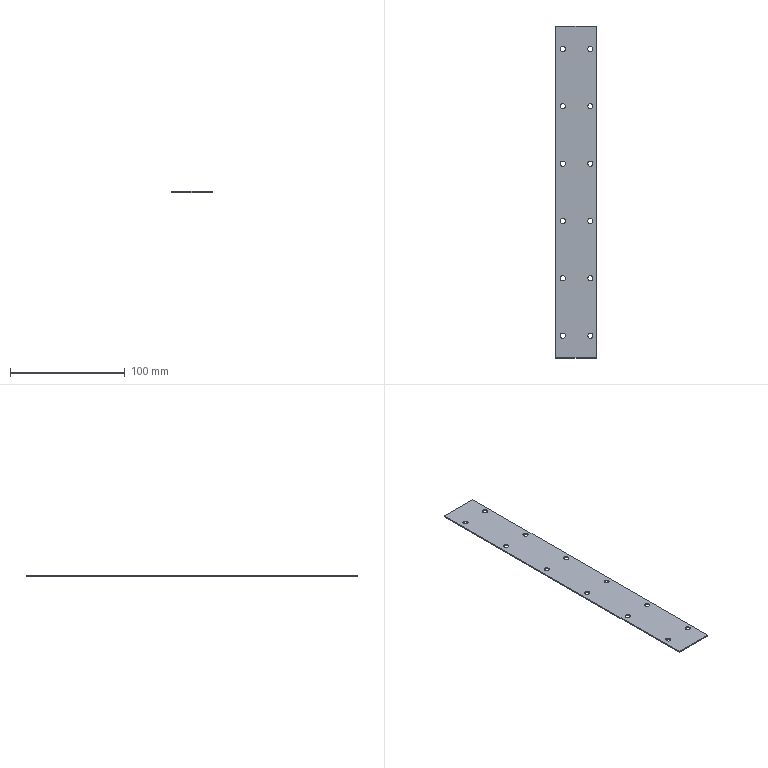Part | STEP file | Conn plate (S) | 1 solid | 30 faces | box 35 x 289.5 x 1 mm | volume 9942 mm3 | cylinder 24 | plane 6 | commonest cylinder face diameters 4.5 x24